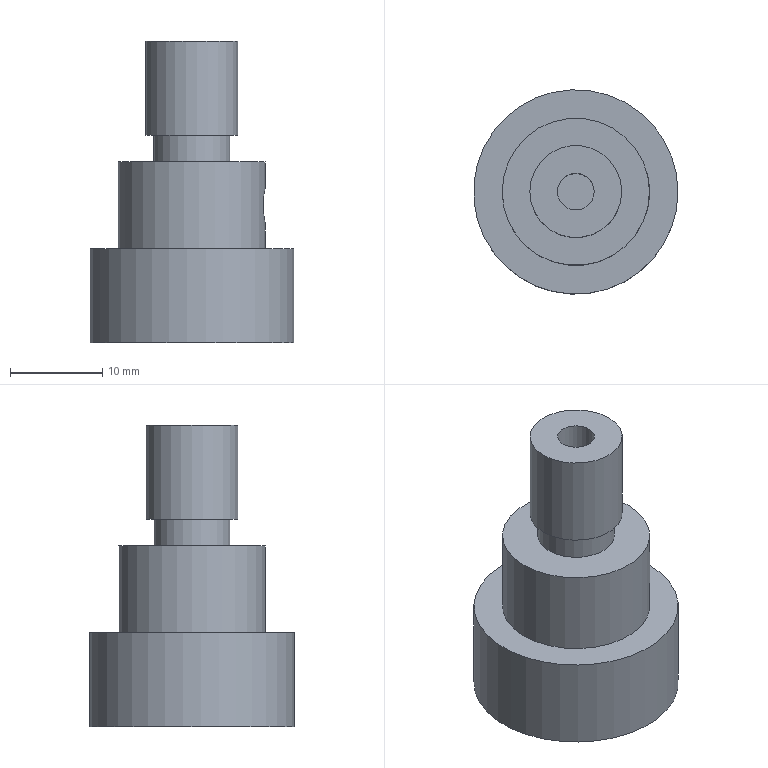Part | NX | features DATUM_CSYS 5, CYLINDER 4, EXTRUDE 4, SKETCH 4, DATUM_PLANE 1, SYMBOLIC_THREAD 1 | 4 solids | 16 faces | box 22.2 x 22.2 x 32.8 mm | volume 6457 mm3 | plane 8 | cylinder 8 | commonest cylinder face diameters 4 x4 8.3 x1 10 x1 16 x1 22.2 x1
STEP:
#1=CARTESIAN_POINT('',(2.,0.,22.54));
#2=VERTEX_POINT('',#1);
#3=CARTESIAN_POINT('',(0.,0.,22.54));
#4=DIRECTION('',(0.,0.,1.));
#5=DIRECTION('',(1.,0.,0.));
#6=AXIS2_PLACEMENT_3D('',#3,#4,#5);
#7=CIRCLE('',#6,2.);
#8=EDGE_CURVE('',#2,#2,#7,.T.);
#9=ORIENTED_EDGE('',*,*,#8,.F.);
#10=EDGE_LOOP('',(#9));
#11=FACE_BOUND('',#10,.T.);
#12=CARTESIAN_POINT('',(4.15,0.,22.54));
#13=VERTEX_POINT('',#12);
#14=CARTESIAN_POINT('',(0.,0.,22.54));
#15=DIRECTION('',(0.,0.,-1.));
#16=DIRECTION('',(1.,0.,0.));
#17=AXIS2_PLACEMENT_3D('',#14,#15,#16);
#18=CIRCLE('',#17,4.15);
#19=EDGE_CURVE('',#13,#13,#18,.T.);
#20=ORIENTED_EDGE('',*,*,#19,.F.);
#21=EDGE_LOOP('',(#20));
#22=FACE_BOUND('',#21,.T.);
#23=CARTESIAN_POINT('',(0.,0.,22.54));
#24=DIRECTION('',(0.,0.,1.));
#25=DIRECTION('',(1.,0.,0.));
#26=AXIS2_PLACEMENT_3D('',#23,#24,#25);
#27=PLANE('',#26);
#28=ADVANCED_FACE('',(#11,#22),#27,.T.);
#29=CARTESIAN_POINT('',(-2.,0.,19.66));
#30=VERTEX_POINT('',#29);
#31=CARTESIAN_POINT('',(0.,0.,19.66));
#32=DIRECTION('',(0.,0.,-1.));
#33=DIRECTION('',(-1.,0.,0.));
#34=AXIS2_PLACEMENT_3D('',#31,#32,#33);
#35=CIRCLE('',#34,2.);
#36=EDGE_CURVE('',#30,#30,#35,.T.);
#37=ORIENTED_EDGE('',*,*,#36,.F.);
#38=EDGE_LOOP('',(#37));
#39=FACE_BOUND('',#38,.T.);
#40=CARTESIAN_POINT('',(4.15,0.,19.66));
#41=VERTEX_POINT('',#40);
#42=CARTESIAN_POINT('',(0.,0.,19.66));
#43=DIRECTION('',(0.,0.,1.));
#44=DIRECTION('',(1.,0.,0.));
#45=AXIS2_PLACEMENT_3D('',#42,#43,#44);
#46=CIRCLE('',#45,4.15);
#47=EDGE_CURVE('',#41,#41,#46,.T.);
#48=ORIENTED_EDGE('',*,*,#47,.F.);
#49=EDGE_LOOP('',(#48));
#50=FACE_BOUND('',#49,.T.);
#51=CARTESIAN_POINT('',(0.,0.,19.66));
#52=DIRECTION('',(0.,0.,-1.));
#53=DIRECTION('',(-1.,0.,0.));
#54=AXIS2_PLACEMENT_3D('',#51,#52,#53);
#55=PLANE('',#54);
#56=ADVANCED_FACE('',(#39,#50),#55,.T.);
#57=ORIENTED_EDGE('',*,*,#19,.T.);
#58=EDGE_LOOP('',(#57));
#59=FACE_BOUND('',#58,.T.);
#60=ORIENTED_EDGE('',*,*,#47,.T.);
#61=EDGE_LOOP('',(#60));
#62=FACE_BOUND('',#61,.T.);
#63=CARTESIAN_POINT('',(0.,0.,19.66));
#64=DIRECTION('',(0.,0.,1.));
#65=DIRECTION('',(1.,0.,0.));
#66=AXIS2_PLACEMENT_3D('',#63,#64,#65);
#67=CYLINDRICAL_SURFACE('',#66,4.15);
#68=ADVANCED_FACE('',(#59,#62),#67,.T.);
#69=ORIENTED_EDGE('',*,*,#36,.T.);
#70=EDGE_LOOP('',(#69));
#71=FACE_BOUND('',#70,.T.);
#72=ORIENTED_EDGE('',*,*,#8,.T.);
#73=EDGE_LOOP('',(#72));
#74=FACE_BOUND('',#73,.T.);
#75=CARTESIAN_POINT('',(0.,0.,4.69));
#76=DIRECTION('',(0.,0.,1.));
#77=DIRECTION('',(1.,0.,0.));
#78=AXIS2_PLACEMENT_3D('',#75,#76,#77);
#79=CYLINDRICAL_SURFACE('',#78,2.);
#80=ADVANCED_FACE('',(#71,#74),#79,.F.);
#81=CLOSED_SHELL('',(#28,#56,#68,#80));
#82=MANIFOLD_SOLID_BREP('',#81);
#83=CARTESIAN_POINT('',(2.,0.,19.66));
#84=VERTEX_POINT('',#83);
#85=CARTESIAN_POINT('',(0.,0.,19.66));
#86=DIRECTION('',(0.,0.,1.));
#87=DIRECTION('',(1.,0.,0.));
#88=AXIS2_PLACEMENT_3D('',#85,#86,#87);
#89=CIRCLE('',#88,2.);
#90=EDGE_CURVE('',#84,#84,#89,.T.);
#91=ORIENTED_EDGE('',*,*,#90,.F.);
#92=EDGE_LOOP('',(#91));
#93=FACE_BOUND('',#92,.T.);
#94=CARTESIAN_POINT('',(8.,0.,19.66));
#95=VERTEX_POINT('',#94);
#96=CARTESIAN_POINT('',(0.,0.,19.66));
#97=DIRECTION('',(0.,0.,-1.));
#98=DIRECTION('',(1.,0.,0.));
#99=AXIS2_PLACEMENT_3D('',#96,#97,#98);
#100=CIRCLE('',#99,8.);
#101=EDGE_CURVE('',#95,#95,#100,.T.);
#102=ORIENTED_EDGE('',*,*,#101,.F.);
#103=EDGE_LOOP('',(#102));
#104=FACE_BOUND('',#103,.T.);
#105=CARTESIAN_POINT('',(0.,0.,19.66));
#106=DIRECTION('',(0.,0.,1.));
#107=DIRECTION('',(1.,0.,0.));
#108=AXIS2_PLACEMENT_3D('',#105,#106,#107);
#109=PLANE('',#108);
#110=ADVANCED_FACE('',(#93,#104),#109,.T.);
#111=CARTESIAN_POINT('',(2.,0.,10.24));
#112=VERTEX_POINT('',#111);
#113=CARTESIAN_POINT('',(0.,0.,10.24));
#114=DIRECTION('',(0.,0.,1.));
#115=DIRECTION('',(1.,0.,0.));
#116=AXIS2_PLACEMENT_3D('',#113,#114,#115);
#117=CIRCLE('',#116,2.);
#118=EDGE_CURVE('',#112,#112,#117,.T.);
#119=ORIENTED_EDGE('',*,*,#118,.T.);
#120=EDGE_LOOP('',(#119));
#121=FACE_BOUND('',#120,.T.);
#122=CARTESIAN_POINT('',(8.,0.,10.24));
#123=VERTEX_POINT('',#122);
#124=CARTESIAN_POINT('',(0.,0.,10.24));
#125=DIRECTION('',(0.,0.,1.));
#126=DIRECTION('',(1.,0.,0.));
#127=AXIS2_PLACEMENT_3D('',#124,#125,#126);
#128=CIRCLE('',#127,8.);
#129=EDGE_CURVE('',#123,#123,#128,.T.);
#130=ORIENTED_EDGE('',*,*,#129,.F.);
#131=EDGE_LOOP('',(#130));
#132=FACE_BOUND('',#131,.T.);
#133=CARTESIAN_POINT('',(0.,0.,10.24));
#134=DIRECTION('',(0.,0.,-1.));
#135=DIRECTION('',(-1.,0.,0.));
#136=AXIS2_PLACEMENT_3D('',#133,#134,#135);
#137=PLANE('',#136);
#138=ADVANCED_FACE('',(#121,#132),#137,.T.);
#139=CARTESIAN_POINT('',(8.,0.,12.95));
#140=VERTEX_POINT('',#139);
#141=CARTESIAN_POINT('',(7.875,-1.569,13.384));
#142=CARTESIAN_POINT('',(8.063,0.0002863,12.733));
#143=CARTESIAN_POINT('',(7.875,1.568,13.384));
#144=CARTESIAN_POINT('',(7.681,2.216,14.948));
#145=CARTESIAN_POINT('',(7.875,1.567,16.518));
#146=CARTESIAN_POINT('',(8.062,0.0009511,17.166));
#147=CARTESIAN_POINT('',(7.875,-1.566,16.519));
#148=CARTESIAN_POINT('',(7.681,-2.216,14.951));
#149=CARTESIAN_POINT('',(7.875,-1.569,13.384));
#150=CARTESIAN_POINT('',(8.063,0.0002863,12.733));
#151=CARTESIAN_POINT('',(7.875,1.568,13.384));
#152=B_SPLINE_CURVE_WITH_KNOTS('',3,(#141,#142,#143,#144,#145,#146,#147,#148,#149,#150,#151),.UNSPECIFIED.,.T.,.F.,(1,1,1,1,1,1,1,1,1,1,1,1,1,1,1),(-0.004708,-0.003139,-0.001569,0.,0.001569,0.003139,0.004708,0.006277,0.007846,0.009416,0.01098,0.01255,0.01412,0.01569,0.01726),.UNSPECIFIED.);
#153=EDGE_CURVE('',#140,#140,#152,.T.);
#154=ORIENTED_EDGE('',*,*,#153,.F.);
#155=EDGE_LOOP('',(#154));
#156=FACE_BOUND('',#155,.T.);
#157=ORIENTED_EDGE('',*,*,#101,.T.);
#158=EDGE_LOOP('',(#157));
#159=FACE_BOUND('',#158,.T.);
#160=ORIENTED_EDGE('',*,*,#129,.T.);
#161=EDGE_LOOP('',(#160));
#162=FACE_BOUND('',#161,.T.);
#163=CARTESIAN_POINT('',(0.,0.,10.24));
#164=DIRECTION('',(0.,0.,1.));
#165=DIRECTION('',(1.,0.,0.));
#166=AXIS2_PLACEMENT_3D('',#163,#164,#165);
#167=CYLINDRICAL_SURFACE('',#166,8.);
#168=ADVANCED_FACE('',(#156,#159,#162),#167,.T.);
#169=ORIENTED_EDGE('',*,*,#153,.T.);
#170=EDGE_LOOP('',(#169));
#171=FACE_BOUND('',#170,.T.);
#172=CARTESIAN_POINT('',(0.,-2.,14.95));
#173=VERTEX_POINT('',#172);
#174=CARTESIAN_POINT('',(0.,2.,14.95));
#175=VERTEX_POINT('',#174);
#176=CARTESIAN_POINT('',(0.,0.,14.95));
#177=DIRECTION('',(0.7071,0.,-0.7071));
#178=DIRECTION('',(0.7071,0.,0.7071));
#179=AXIS2_PLACEMENT_3D('',#176,#177,#178);
#180=ELLIPSE('',#179,2.828,2.);
#181=EDGE_CURVE('',#173,#175,#180,.F.);
#182=ORIENTED_EDGE('',*,*,#181,.T.);
#183=CARTESIAN_POINT('',(0.,0.,14.95));
#184=DIRECTION('',(0.7071,0.,0.7071));
#185=DIRECTION('',(0.7071,0.,-0.7071));
#186=AXIS2_PLACEMENT_3D('',#183,#184,#185);
#187=ELLIPSE('',#186,2.828,2.);
#188=EDGE_CURVE('',#175,#173,#187,.F.);
#189=ORIENTED_EDGE('',*,*,#188,.T.);
#190=EDGE_LOOP('',(#182,#189));
#191=FACE_BOUND('',#190,.T.);
#192=CARTESIAN_POINT('',(0.,0.,14.95));
#193=DIRECTION('',(1.,0.,0.));
#194=DIRECTION('',(0.,0.,-1.));
#195=AXIS2_PLACEMENT_3D('',#192,#193,#194);
#196=CYLINDRICAL_SURFACE('',#195,2.);
#197=ADVANCED_FACE('',(#171,#191),#196,.F.);
#198=ORIENTED_EDGE('',*,*,#118,.F.);
#199=EDGE_LOOP('',(#198));
#200=FACE_BOUND('',#199,.T.);
#201=ORIENTED_EDGE('',*,*,#90,.T.);
#202=EDGE_LOOP('',(#201));
#203=FACE_BOUND('',#202,.T.);
#204=ORIENTED_EDGE('',*,*,#181,.F.);
#205=ORIENTED_EDGE('',*,*,#188,.F.);
#206=EDGE_LOOP('',(#204,#205));
#207=FACE_BOUND('',#206,.T.);
#208=CARTESIAN_POINT('',(0.,0.,10.24));
#209=DIRECTION('',(0.,0.,1.));
#210=DIRECTION('',(1.,0.,0.));
#211=AXIS2_PLACEMENT_3D('',#208,#209,#210);
#212=CYLINDRICAL_SURFACE('',#211,2.);
#213=ADVANCED_FACE('',(#200,#203,#207),#212,.F.);
#214=CLOSED_SHELL('',(#110,#138,#168,#197,#213));
#215=MANIFOLD_SOLID_BREP('',#214);
#216=CARTESIAN_POINT('',(2.,0.,32.8));
#217=VERTEX_POINT('',#216);
#218=CARTESIAN_POINT('',(0.,0.,32.8));
#219=DIRECTION('',(0.,0.,1.));
#220=DIRECTION('',(1.,0.,0.));
#221=AXIS2_PLACEMENT_3D('',#218,#219,#220);
#222=CIRCLE('',#221,2.);
#223=EDGE_CURVE('',#217,#217,#222,.T.);
#224=ORIENTED_EDGE('',*,*,#223,.F.);
#225=EDGE_LOOP('',(#224));
#226=FACE_BOUND('',#225,.T.);
#227=CARTESIAN_POINT('',(5.,0.,32.8));
#228=VERTEX_POINT('',#227);
#229=CARTESIAN_POINT('',(0.,0.,32.8));
#230=DIRECTION('',(0.,0.,-1.));
#231=DIRECTION('',(1.,0.,0.));
#232=AXIS2_PLACEMENT_3D('',#229,#230,#231);
#233=CIRCLE('',#232,5.);
#234=EDGE_CURVE('',#228,#228,#233,.T.);
#235=ORIENTED_EDGE('',*,*,#234,.F.);
#236=EDGE_LOOP('',(#235));
#237=FACE_BOUND('',#236,.T.);
#238=CARTESIAN_POINT('',(0.,0.,32.8));
#239=DIRECTION('',(0.,0.,1.));
#240=DIRECTION('',(1.,0.,0.));
#241=AXIS2_PLACEMENT_3D('',#238,#239,#240);
#242=PLANE('',#241);
#243=ADVANCED_FACE('',(#226,#237),#242,.T.);
#244=CARTESIAN_POINT('',(-2.,0.,22.54));
#245=VERTEX_POINT('',#244);
#246=CARTESIAN_POINT('',(0.,0.,22.54));
#247=DIRECTION('',(0.,0.,-1.));
#248=DIRECTION('',(-1.,0.,0.));
#249=AXIS2_PLACEMENT_3D('',#246,#247,#248);
#250=CIRCLE('',#249,2.);
#251=EDGE_CURVE('',#245,#245,#250,.T.);
#252=ORIENTED_EDGE('',*,*,#251,.F.);
#253=EDGE_LOOP('',(#252));
#254=FACE_BOUND('',#253,.T.);
#255=CARTESIAN_POINT('',(5.,0.,22.54));
#256=VERTEX_POINT('',#255);
#257=CARTESIAN_POINT('',(0.,0.,22.54));
#258=DIRECTION('',(0.,0.,1.));
#259=DIRECTION('',(1.,0.,0.));
#260=AXIS2_PLACEMENT_3D('',#257,#258,#259);
#261=CIRCLE('',#260,5.);
#262=EDGE_CURVE('',#256,#256,#261,.T.);
#263=ORIENTED_EDGE('',*,*,#262,.F.);
#264=EDGE_LOOP('',(#263));
#265=FACE_BOUND('',#264,.T.);
#266=CARTESIAN_POINT('',(0.,0.,22.54));
#267=DIRECTION('',(0.,0.,-1.));
#268=DIRECTION('',(-1.,0.,0.));
#269=AXIS2_PLACEMENT_3D('',#266,#267,#268);
#270=PLANE('',#269);
#271=ADVANCED_FACE('',(#254,#265),#270,.T.);
#272=ORIENTED_EDGE('',*,*,#234,.T.);
#273=EDGE_LOOP('',(#272));
#274=FACE_BOUND('',#273,.T.);
#275=ORIENTED_EDGE('',*,*,#262,.T.);
#276=EDGE_LOOP('',(#275));
#277=FACE_BOUND('',#276,.T.);
#278=CARTESIAN_POINT('',(0.,0.,22.54));
#279=DIRECTION('',(0.,0.,1.));
#280=DIRECTION('',(1.,0.,0.));
#281=AXIS2_PLACEMENT_3D('',#278,#279,#280);
#282=CYLINDRICAL_SURFACE('',#281,5.);
#283=ADVANCED_FACE('',(#274,#277),#282,.T.);
#284=ORIENTED_EDGE('',*,*,#251,.T.);
#285=EDGE_LOOP('',(#284));
#286=FACE_BOUND('',#285,.T.);
#287=ORIENTED_EDGE('',*,*,#223,.T.);
#288=EDGE_LOOP('',(#287));
#289=FACE_BOUND('',#288,.T.);
#290=CARTESIAN_POINT('',(0.,0.,14.95));
#291=DIRECTION('',(0.,0.,1.));
#292=DIRECTION('',(1.,0.,0.));
#293=AXIS2_PLACEMENT_3D('',#290,#291,#292);
#294=CYLINDRICAL_SURFACE('',#293,2.);
#295=ADVANCED_FACE('',(#286,#289),#294,.F.);
#296=CLOSED_SHELL('',(#243,#271,#283,#295));
#297=MANIFOLD_SOLID_BREP('',#296);
#298=CARTESIAN_POINT('',(11.1,0.,10.24));
#299=VERTEX_POINT('',#298);
#300=CARTESIAN_POINT('',(0.,0.,10.24));
#301=DIRECTION('',(0.,0.,-1.));
#302=DIRECTION('',(1.,0.,0.));
#303=AXIS2_PLACEMENT_3D('',#300,#301,#302);
#304=CIRCLE('',#303,11.1);
#305=EDGE_CURVE('',#299,#299,#304,.T.);
#306=ORIENTED_EDGE('',*,*,#305,.F.);
#307=EDGE_LOOP('',(#306));
#308=FACE_BOUND('',#307,.T.);
#309=CARTESIAN_POINT('',(0.,0.,10.24));
#310=DIRECTION('',(0.,0.,1.));
#311=DIRECTION('',(1.,0.,0.));
#312=AXIS2_PLACEMENT_3D('',#309,#310,#311);
#313=PLANE('',#312);
#314=ADVANCED_FACE('',(#308),#313,.T.);
#315=CARTESIAN_POINT('',(11.1,0.,0.));
#316=VERTEX_POINT('',#315);
#317=CARTESIAN_POINT('',(0.,0.,0.));
#318=DIRECTION('',(0.,0.,1.));
#319=DIRECTION('',(1.,0.,0.));
#320=AXIS2_PLACEMENT_3D('',#317,#318,#319);
#321=CIRCLE('',#320,11.1);
#322=EDGE_CURVE('',#316,#316,#321,.T.);
#323=ORIENTED_EDGE('',*,*,#322,.F.);
#324=EDGE_LOOP('',(#323));
#325=FACE_BOUND('',#324,.T.);
#326=CARTESIAN_POINT('',(0.,0.,0.));
#327=DIRECTION('',(0.,0.,-1.));
#328=DIRECTION('',(-1.,0.,0.));
#329=AXIS2_PLACEMENT_3D('',#326,#327,#328);
#330=PLANE('',#329);
#331=ADVANCED_FACE('',(#325),#330,.T.);
#332=ORIENTED_EDGE('',*,*,#305,.T.);
#333=EDGE_LOOP('',(#332));
#334=FACE_BOUND('',#333,.T.);
#335=ORIENTED_EDGE('',*,*,#322,.T.);
#336=EDGE_LOOP('',(#335));
#337=FACE_BOUND('',#336,.T.);
#338=CARTESIAN_POINT('',(0.,0.,0.));
#339=DIRECTION('',(0.,0.,1.));
#340=DIRECTION('',(1.,0.,0.));
#341=AXIS2_PLACEMENT_3D('',#338,#339,#340);
#342=CYLINDRICAL_SURFACE('',#341,11.1);
#343=ADVANCED_FACE('',(#334,#337),#342,.T.);
#344=CLOSED_SHELL('',(#314,#331,#343));
#345=MANIFOLD_SOLID_BREP('',#344);
#346=(LENGTH_UNIT()NAMED_UNIT(*)SI_UNIT(.MILLI.,.METRE.));
#347=UNCERTAINTY_MEASURE_WITH_UNIT(LENGTH_MEASURE(0.0508),#346,'','');
#348=(NAMED_UNIT(*)PLANE_ANGLE_UNIT()SI_UNIT($,.RADIAN.));
#349=(NAMED_UNIT(*)SI_UNIT($,.STERADIAN.)SOLID_ANGLE_UNIT());
#350=(GEOMETRIC_REPRESENTATION_CONTEXT(3)GLOBAL_UNCERTAINTY_ASSIGNED_CONTEXT((#347))GLOBAL_UNIT_ASSIGNED_CONTEXT((#346,#348,#349))REPRESENTATION_CONTEXT('',''));
#351=ADVANCED_BREP_SHAPE_REPRESENTATION('',(#82,#215,#297,#345),#350);